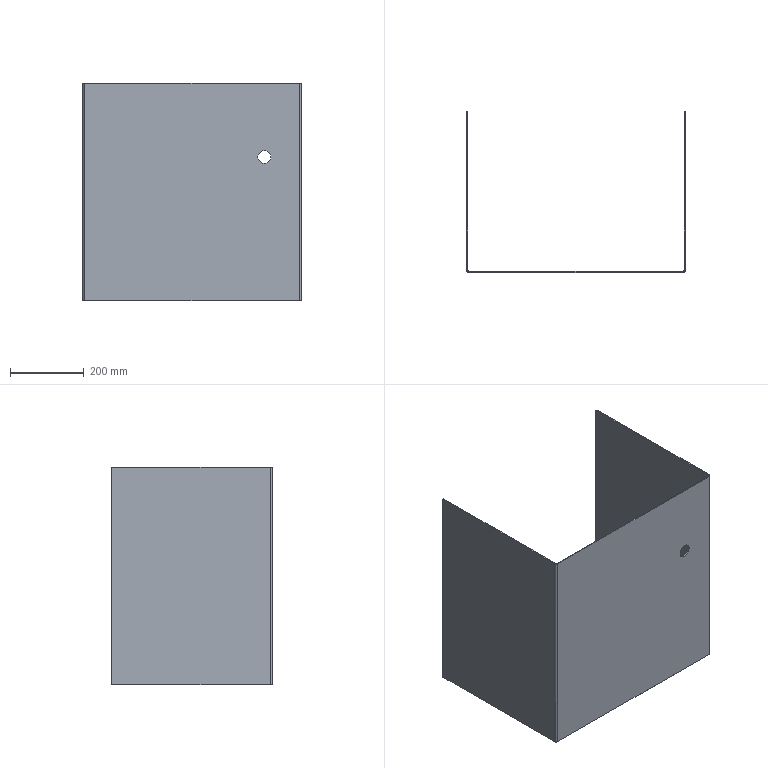Part | SolidWorks | features ICE 2, FlatPattern 1, SMBaseFlange 1, SheetMetal 1 | 1 solid | 28 faces | box 592 x 437 x 590 mm | volume 2574453 mm3 | plane 18 | cylinder 10 | commonest cylinder face diameters 6 x6 12 x2 35 x2
STEP:
#1=CARTESIAN_POINT('',(492.,0.,372.5));
#2=VERTEX_POINT('',#1);
#3=CARTESIAN_POINT('',(492.,0.,407.5));
#4=VERTEX_POINT('',#3);
#5=CARTESIAN_POINT('',(492.,0.,390.));
#6=DIRECTION('',(0.,1.,0.));
#7=DIRECTION('',(0.,0.,1.));
#8=AXIS2_PLACEMENT_3D('',#5,#6,#7);
#9=CIRCLE('',#8,17.5);
#10=EDGE_CURVE('',#2,#4,#9,.T.);
#11=ORIENTED_EDGE('',*,*,#10,.F.);
#12=CARTESIAN_POINT('',(492.,3.,372.5));
#13=VERTEX_POINT('',#12);
#14=CARTESIAN_POINT('',(492.,-7.,372.5));
#15=DIRECTION('',(0.,1.,0.));
#16=VECTOR('',#15,1000.);
#17=LINE('',#14,#16);
#18=EDGE_CURVE('',#2,#13,#17,.T.);
#19=ORIENTED_EDGE('',*,*,#18,.T.);
#20=CARTESIAN_POINT('',(492.,3.,407.5));
#21=VERTEX_POINT('',#20);
#22=CARTESIAN_POINT('',(492.,3.,390.));
#23=DIRECTION('',(0.,1.,0.));
#24=DIRECTION('',(0.,0.,1.));
#25=AXIS2_PLACEMENT_3D('',#22,#23,#24);
#26=CIRCLE('',#25,17.5);
#27=EDGE_CURVE('',#13,#21,#26,.T.);
#28=ORIENTED_EDGE('',*,*,#27,.T.);
#29=CARTESIAN_POINT('',(492.,-7.,407.5));
#30=DIRECTION('',(0.,1.,0.));
#31=VECTOR('',#30,1000.);
#32=LINE('',#29,#31);
#33=EDGE_CURVE('',#4,#21,#32,.T.);
#34=ORIENTED_EDGE('',*,*,#33,.F.);
#35=EDGE_LOOP('',(#11,#19,#28,#34));
#36=FACE_OUTER_BOUND('',#35,.T.);
#37=CARTESIAN_POINT('',(492.,-7.,390.));
#38=DIRECTION('',(0.,1.,0.));
#39=DIRECTION('',(0.,0.,1.));
#40=AXIS2_PLACEMENT_3D('',#37,#38,#39);
#41=CYLINDRICAL_SURFACE('',#40,17.5);
#42=ADVANCED_FACE('',(#36),#41,.F.);
#43=CARTESIAN_POINT('',(592.,434.,0.));
#44=VERTEX_POINT('',#43);
#45=CARTESIAN_POINT('',(592.,437.,3.));
#46=VERTEX_POINT('',#45);
#47=CARTESIAN_POINT('',(592.,434.,3.));
#48=DIRECTION('',(1.,0.,0.));
#49=DIRECTION('',(0.,0.,1.));
#50=AXIS2_PLACEMENT_3D('',#47,#48,#49);
#51=CIRCLE('',#50,3.);
#52=EDGE_CURVE('',#44,#46,#51,.T.);
#53=ORIENTED_EDGE('',*,*,#52,.T.);
#54=CARTESIAN_POINT('',(592.,437.,587.));
#55=VERTEX_POINT('',#54);
#56=CARTESIAN_POINT('',(592.,437.,590.));
#57=DIRECTION('',(0.,0.,-1.));
#58=VECTOR('',#57,1000.);
#59=LINE('',#56,#58);
#60=EDGE_CURVE('',#55,#46,#59,.T.);
#61=ORIENTED_EDGE('',*,*,#60,.F.);
#62=CARTESIAN_POINT('',(592.,434.,590.));
#63=VERTEX_POINT('',#62);
#64=CARTESIAN_POINT('',(592.,434.,587.));
#65=DIRECTION('',(1.,0.,0.));
#66=DIRECTION('',(0.,0.,1.));
#67=AXIS2_PLACEMENT_3D('',#64,#65,#66);
#68=CIRCLE('',#67,3.);
#69=EDGE_CURVE('',#55,#63,#68,.T.);
#70=ORIENTED_EDGE('',*,*,#69,.T.);
#71=CARTESIAN_POINT('',(592.,6.,590.));
#72=VERTEX_POINT('',#71);
#73=CARTESIAN_POINT('',(592.,0.,590.));
#74=DIRECTION('',(0.,1.,0.));
#75=VECTOR('',#74,1000.);
#76=LINE('',#73,#75);
#77=EDGE_CURVE('',#72,#63,#76,.T.);
#78=ORIENTED_EDGE('',*,*,#77,.F.);
#79=CARTESIAN_POINT('',(592.,6.,0.));
#80=VERTEX_POINT('',#79);
#81=CARTESIAN_POINT('',(592.,6.,590.));
#82=DIRECTION('',(0.,0.,-1.));
#83=VECTOR('',#82,1000.);
#84=LINE('',#81,#83);
#85=EDGE_CURVE('',#72,#80,#84,.T.);
#86=ORIENTED_EDGE('',*,*,#85,.T.);
#87=CARTESIAN_POINT('',(592.,0.,0.));
#88=DIRECTION('',(0.,1.,0.));
#89=VECTOR('',#88,1000.);
#90=LINE('',#87,#89);
#91=EDGE_CURVE('',#80,#44,#90,.T.);
#92=ORIENTED_EDGE('',*,*,#91,.T.);
#93=EDGE_LOOP('',(#53,#61,#70,#78,#86,#92));
#94=FACE_OUTER_BOUND('',#93,.T.);
#95=CARTESIAN_POINT('',(592.,0.,590.));
#96=DIRECTION('',(-1.,0.,0.));
#97=DIRECTION('',(0.,0.,1.));
#98=AXIS2_PLACEMENT_3D('',#95,#96,#97);
#99=PLANE('',#98);
#100=ADVANCED_FACE('',(#94),#99,.F.);
#101=CARTESIAN_POINT('',(589.,437.,587.));
#102=VERTEX_POINT('',#101);
#103=CARTESIAN_POINT('',(589.,437.,3.));
#104=VERTEX_POINT('',#103);
#105=CARTESIAN_POINT('',(589.,437.,590.));
#106=DIRECTION('',(0.,0.,-1.));
#107=VECTOR('',#106,1000.);
#108=LINE('',#105,#107);
#109=EDGE_CURVE('',#102,#104,#108,.T.);
#110=ORIENTED_EDGE('',*,*,#109,.T.);
#111=CARTESIAN_POINT('',(589.,434.,0.));
#112=VERTEX_POINT('',#111);
#113=CARTESIAN_POINT('',(589.,434.,3.));
#114=DIRECTION('',(1.,0.,0.));
#115=DIRECTION('',(0.,0.,1.));
#116=AXIS2_PLACEMENT_3D('',#113,#114,#115);
#117=CIRCLE('',#116,3.);
#118=EDGE_CURVE('',#112,#104,#117,.T.);
#119=ORIENTED_EDGE('',*,*,#118,.F.);
#120=CARTESIAN_POINT('',(589.,6.,0.));
#121=VERTEX_POINT('',#120);
#122=CARTESIAN_POINT('',(589.,0.,0.));
#123=DIRECTION('',(0.,1.,0.));
#124=VECTOR('',#123,1000.);
#125=LINE('',#122,#124);
#126=EDGE_CURVE('',#121,#112,#125,.T.);
#127=ORIENTED_EDGE('',*,*,#126,.F.);
#128=CARTESIAN_POINT('',(589.,6.,590.));
#129=VERTEX_POINT('',#128);
#130=CARTESIAN_POINT('',(589.,6.,590.));
#131=DIRECTION('',(0.,0.,-1.));
#132=VECTOR('',#131,1000.);
#133=LINE('',#130,#132);
#134=EDGE_CURVE('',#129,#121,#133,.T.);
#135=ORIENTED_EDGE('',*,*,#134,.F.);
#136=CARTESIAN_POINT('',(589.,434.,590.));
#137=VERTEX_POINT('',#136);
#138=CARTESIAN_POINT('',(589.,0.,590.));
#139=DIRECTION('',(0.,1.,0.));
#140=VECTOR('',#139,1000.);
#141=LINE('',#138,#140);
#142=EDGE_CURVE('',#129,#137,#141,.T.);
#143=ORIENTED_EDGE('',*,*,#142,.T.);
#144=CARTESIAN_POINT('',(589.,434.,587.));
#145=DIRECTION('',(1.,0.,0.));
#146=DIRECTION('',(0.,0.,1.));
#147=AXIS2_PLACEMENT_3D('',#144,#145,#146);
#148=CIRCLE('',#147,3.);
#149=EDGE_CURVE('',#102,#137,#148,.T.);
#150=ORIENTED_EDGE('',*,*,#149,.F.);
#151=EDGE_LOOP('',(#110,#119,#127,#135,#143,#150));
#152=FACE_OUTER_BOUND('',#151,.T.);
#153=CARTESIAN_POINT('',(589.,0.,590.));
#154=DIRECTION('',(-1.,0.,0.));
#155=DIRECTION('',(0.,0.,1.));
#156=AXIS2_PLACEMENT_3D('',#153,#154,#155);
#157=PLANE('',#156);
#158=ADVANCED_FACE('',(#152),#157,.T.);
#159=ORIENTED_EDGE('',*,*,#60,.T.);
#160=CARTESIAN_POINT('',(589.,437.,3.));
#161=DIRECTION('',(1.,0.,0.));
#162=VECTOR('',#161,1000.);
#163=LINE('',#160,#162);
#164=EDGE_CURVE('',#104,#46,#163,.T.);
#165=ORIENTED_EDGE('',*,*,#164,.F.);
#166=ORIENTED_EDGE('',*,*,#109,.F.);
#167=CARTESIAN_POINT('',(589.,437.,587.));
#168=DIRECTION('',(1.,0.,0.));
#169=VECTOR('',#168,1000.);
#170=LINE('',#167,#169);
#171=EDGE_CURVE('',#102,#55,#170,.T.);
#172=ORIENTED_EDGE('',*,*,#171,.T.);
#173=EDGE_LOOP('',(#159,#165,#166,#172));
#174=FACE_OUTER_BOUND('',#173,.T.);
#175=CARTESIAN_POINT('',(589.,437.,590.));
#176=DIRECTION('',(0.,1.,0.));
#177=DIRECTION('',(0.,0.,1.));
#178=AXIS2_PLACEMENT_3D('',#175,#176,#177);
#179=PLANE('',#178);
#180=ADVANCED_FACE('',(#174),#179,.T.);
#181=CARTESIAN_POINT('',(3.,434.,0.));
#182=VERTEX_POINT('',#181);
#183=CARTESIAN_POINT('',(3.,6.,0.));
#184=VERTEX_POINT('',#183);
#185=CARTESIAN_POINT('',(3.,0.,0.));
#186=DIRECTION('',(0.,-1.,0.));
#187=VECTOR('',#186,1000.);
#188=LINE('',#185,#187);
#189=EDGE_CURVE('',#182,#184,#188,.T.);
#190=ORIENTED_EDGE('',*,*,#189,.F.);
#191=CARTESIAN_POINT('',(3.,437.,3.));
#192=VERTEX_POINT('',#191);
#193=CARTESIAN_POINT('',(3.,434.,3.));
#194=DIRECTION('',(-1.,0.,0.));
#195=DIRECTION('',(0.,0.,-1.));
#196=AXIS2_PLACEMENT_3D('',#193,#194,#195);
#197=CIRCLE('',#196,3.);
#198=EDGE_CURVE('',#192,#182,#197,.T.);
#199=ORIENTED_EDGE('',*,*,#198,.F.);
#200=CARTESIAN_POINT('',(3.,437.,587.));
#201=VERTEX_POINT('',#200);
#202=CARTESIAN_POINT('',(3.,437.,590.));
#203=DIRECTION('',(0.,0.,-1.));
#204=VECTOR('',#203,1000.);
#205=LINE('',#202,#204);
#206=EDGE_CURVE('',#201,#192,#205,.T.);
#207=ORIENTED_EDGE('',*,*,#206,.F.);
#208=CARTESIAN_POINT('',(3.,434.,590.));
#209=VERTEX_POINT('',#208);
#210=CARTESIAN_POINT('',(3.,434.,587.));
#211=DIRECTION('',(-1.,0.,0.));
#212=DIRECTION('',(0.,0.,-1.));
#213=AXIS2_PLACEMENT_3D('',#210,#211,#212);
#214=CIRCLE('',#213,3.);
#215=EDGE_CURVE('',#209,#201,#214,.T.);
#216=ORIENTED_EDGE('',*,*,#215,.F.);
#217=CARTESIAN_POINT('',(3.,6.,590.));
#218=VERTEX_POINT('',#217);
#219=CARTESIAN_POINT('',(3.,0.,590.));
#220=DIRECTION('',(0.,-1.,0.));
#221=VECTOR('',#220,1000.);
#222=LINE('',#219,#221);
#223=EDGE_CURVE('',#209,#218,#222,.T.);
#224=ORIENTED_EDGE('',*,*,#223,.T.);
#225=CARTESIAN_POINT('',(3.,6.,590.));
#226=DIRECTION('',(0.,0.,-1.));
#227=VECTOR('',#226,1000.);
#228=LINE('',#225,#227);
#229=EDGE_CURVE('',#218,#184,#228,.T.);
#230=ORIENTED_EDGE('',*,*,#229,.T.);
#231=EDGE_LOOP('',(#190,#199,#207,#216,#224,#230));
#232=FACE_OUTER_BOUND('',#231,.T.);
#233=CARTESIAN_POINT('',(3.,0.,590.));
#234=DIRECTION('',(1.,0.,0.));
#235=DIRECTION('',(0.,0.,-1.));
#236=AXIS2_PLACEMENT_3D('',#233,#234,#235);
#237=PLANE('',#236);
#238=ADVANCED_FACE('',(#232),#237,.T.);
#239=CARTESIAN_POINT('',(0.,437.,3.));
#240=VERTEX_POINT('',#239);
#241=CARTESIAN_POINT('',(0.,434.,0.));
#242=VERTEX_POINT('',#241);
#243=CARTESIAN_POINT('',(0.,434.,3.));
#244=DIRECTION('',(-1.,0.,0.));
#245=DIRECTION('',(0.,0.,-1.));
#246=AXIS2_PLACEMENT_3D('',#243,#244,#245);
#247=CIRCLE('',#246,3.);
#248=EDGE_CURVE('',#240,#242,#247,.T.);
#249=ORIENTED_EDGE('',*,*,#248,.T.);
#250=CARTESIAN_POINT('',(0.,6.,0.));
#251=VERTEX_POINT('',#250);
#252=CARTESIAN_POINT('',(0.,0.,0.));
#253=DIRECTION('',(0.,-1.,0.));
#254=VECTOR('',#253,1000.);
#255=LINE('',#252,#254);
#256=EDGE_CURVE('',#242,#251,#255,.T.);
#257=ORIENTED_EDGE('',*,*,#256,.T.);
#258=CARTESIAN_POINT('',(0.,6.,590.));
#259=VERTEX_POINT('',#258);
#260=CARTESIAN_POINT('',(0.,6.,590.));
#261=DIRECTION('',(0.,0.,-1.));
#262=VECTOR('',#261,1000.);
#263=LINE('',#260,#262);
#264=EDGE_CURVE('',#259,#251,#263,.T.);
#265=ORIENTED_EDGE('',*,*,#264,.F.);
#266=CARTESIAN_POINT('',(0.,434.,590.));
#267=VERTEX_POINT('',#266);
#268=CARTESIAN_POINT('',(0.,0.,590.));
#269=DIRECTION('',(0.,-1.,0.));
#270=VECTOR('',#269,1000.);
#271=LINE('',#268,#270);
#272=EDGE_CURVE('',#267,#259,#271,.T.);
#273=ORIENTED_EDGE('',*,*,#272,.F.);
#274=CARTESIAN_POINT('',(0.,437.,587.));
#275=VERTEX_POINT('',#274);
#276=CARTESIAN_POINT('',(0.,434.,587.));
#277=DIRECTION('',(-1.,0.,0.));
#278=DIRECTION('',(0.,0.,-1.));
#279=AXIS2_PLACEMENT_3D('',#276,#277,#278);
#280=CIRCLE('',#279,3.);
#281=EDGE_CURVE('',#267,#275,#280,.T.);
#282=ORIENTED_EDGE('',*,*,#281,.T.);
#283=CARTESIAN_POINT('',(0.,437.,590.));
#284=DIRECTION('',(0.,0.,-1.));
#285=VECTOR('',#284,1000.);
#286=LINE('',#283,#285);
#287=EDGE_CURVE('',#275,#240,#286,.T.);
#288=ORIENTED_EDGE('',*,*,#287,.T.);
#289=EDGE_LOOP('',(#249,#257,#265,#273,#282,#288));
#290=FACE_OUTER_BOUND('',#289,.T.);
#291=CARTESIAN_POINT('',(0.,0.,590.));
#292=DIRECTION('',(1.,0.,0.));
#293=DIRECTION('',(0.,0.,-1.));
#294=AXIS2_PLACEMENT_3D('',#291,#292,#293);
#295=PLANE('',#294);
#296=ADVANCED_FACE('',(#290),#295,.F.);
#297=ORIENTED_EDGE('',*,*,#77,.T.);
#298=CARTESIAN_POINT('',(589.,434.,590.));
#299=DIRECTION('',(1.,0.,0.));
#300=VECTOR('',#299,1000.);
#301=LINE('',#298,#300);
#302=EDGE_CURVE('',#137,#63,#301,.T.);
#303=ORIENTED_EDGE('',*,*,#302,.F.);
#304=ORIENTED_EDGE('',*,*,#142,.F.);
#305=CARTESIAN_POINT('',(589.,6.,590.));
#306=DIRECTION('',(1.,0.,0.));
#307=VECTOR('',#306,1000.);
#308=LINE('',#305,#307);
#309=EDGE_CURVE('',#129,#72,#308,.T.);
#310=ORIENTED_EDGE('',*,*,#309,.T.);
#311=EDGE_LOOP('',(#297,#303,#304,#310));
#312=FACE_OUTER_BOUND('',#311,.T.);
#313=CARTESIAN_POINT('',(586.,6.,590.));
#314=DIRECTION('',(0.,0.,1.));
#315=DIRECTION('',(1.,0.,0.));
#316=AXIS2_PLACEMENT_3D('',#313,#314,#315);
#317=PLANE('',#316);
#318=ADVANCED_FACE('',(#312),#317,.T.);
#319=CARTESIAN_POINT('',(3.,437.,3.));
#320=DIRECTION('',(-1.,0.,0.));
#321=VECTOR('',#320,1000.);
#322=LINE('',#319,#321);
#323=EDGE_CURVE('',#192,#240,#322,.T.);
#324=ORIENTED_EDGE('',*,*,#323,.T.);
#325=ORIENTED_EDGE('',*,*,#287,.F.);
#326=CARTESIAN_POINT('',(3.,437.,587.));
#327=DIRECTION('',(-1.,0.,0.));
#328=VECTOR('',#327,1000.);
#329=LINE('',#326,#328);
#330=EDGE_CURVE('',#201,#275,#329,.T.);
#331=ORIENTED_EDGE('',*,*,#330,.F.);
#332=ORIENTED_EDGE('',*,*,#206,.T.);
#333=EDGE_LOOP('',(#324,#325,#331,#332));
#334=FACE_OUTER_BOUND('',#333,.T.);
#335=CARTESIAN_POINT('',(0.,437.,590.));
#336=DIRECTION('',(0.,1.,0.));
#337=DIRECTION('',(0.,0.,1.));
#338=AXIS2_PLACEMENT_3D('',#335,#336,#337);
#339=PLANE('',#338);
#340=ADVANCED_FACE('',(#334),#339,.T.);
#341=CARTESIAN_POINT('',(0.,6.,590.));
#342=DIRECTION('',(1.,0.,0.));
#343=VECTOR('',#342,1000.);
#344=LINE('',#341,#343);
#345=EDGE_CURVE('',#259,#218,#344,.T.);
#346=ORIENTED_EDGE('',*,*,#345,.F.);
#347=CARTESIAN_POINT('',(6.,0.,590.));
#348=VERTEX_POINT('',#347);
#349=CARTESIAN_POINT('',(6.,6.,590.));
#350=DIRECTION('',(0.,0.,1.));
#351=DIRECTION('',(-1.,0.,0.));
#352=AXIS2_PLACEMENT_3D('',#349,#350,#351);
#353=CIRCLE('',#352,6.);
#354=EDGE_CURVE('',#259,#348,#353,.T.);
#355=ORIENTED_EDGE('',*,*,#354,.T.);
#356=CARTESIAN_POINT('',(6.,3.,590.));
#357=VERTEX_POINT('',#356);
#358=CARTESIAN_POINT('',(6.,3.,590.));
#359=DIRECTION('',(0.,-1.,0.));
#360=VECTOR('',#359,1000.);
#361=LINE('',#358,#360);
#362=EDGE_CURVE('',#357,#348,#361,.T.);
#363=ORIENTED_EDGE('',*,*,#362,.F.);
#364=CARTESIAN_POINT('',(6.,6.,590.));
#365=DIRECTION('',(0.,0.,1.));
#366=DIRECTION('',(1.,0.,0.));
#367=AXIS2_PLACEMENT_3D('',#364,#365,#366);
#368=CIRCLE('',#367,3.);
#369=EDGE_CURVE('',#218,#357,#368,.T.);
#370=ORIENTED_EDGE('',*,*,#369,.F.);
#371=EDGE_LOOP('',(#346,#355,#363,#370));
#372=FACE_OUTER_BOUND('',#371,.T.);
#373=CARTESIAN_POINT('',(0.,6.,590.));
#374=DIRECTION('',(0.,0.,1.));
#375=DIRECTION('',(1.,0.,0.));
#376=AXIS2_PLACEMENT_3D('',#373,#374,#375);
#377=PLANE('',#376);
#378=ADVANCED_FACE('',(#372),#377,.T.);
#379=CARTESIAN_POINT('',(3.,434.,590.));
#380=DIRECTION('',(-1.,0.,0.));
#381=VECTOR('',#380,1000.);
#382=LINE('',#379,#381);
#383=EDGE_CURVE('',#209,#267,#382,.T.);
#384=ORIENTED_EDGE('',*,*,#383,.T.);
#385=ORIENTED_EDGE('',*,*,#272,.T.);
#386=ORIENTED_EDGE('',*,*,#345,.T.);
#387=ORIENTED_EDGE('',*,*,#223,.F.);
#388=EDGE_LOOP('',(#384,#385,#386,#387));
#389=FACE_OUTER_BOUND('',#388,.T.);
#390=CARTESIAN_POINT('',(6.,3.,590.));
#391=DIRECTION('',(0.,0.,1.));
#392=DIRECTION('',(1.,0.,0.));
#393=AXIS2_PLACEMENT_3D('',#390,#391,#392);
#394=PLANE('',#393);
#395=ADVANCED_FACE('',(#389),#394,.T.);
#396=CARTESIAN_POINT('',(6.,0.,0.));
#397=VERTEX_POINT('',#396);
#398=CARTESIAN_POINT('',(6.,3.,0.));
#399=VERTEX_POINT('',#398);
#400=CARTESIAN_POINT('',(6.,0.,0.));
#401=DIRECTION('',(0.,1.,0.));
#402=VECTOR('',#401,1000.);
#403=LINE('',#400,#402);
#404=EDGE_CURVE('',#397,#399,#403,.T.);
#405=ORIENTED_EDGE('',*,*,#404,.F.);
#406=CARTESIAN_POINT('',(6.,6.,0.));
#407=DIRECTION('',(0.,0.,1.));
#408=DIRECTION('',(-1.,0.,0.));
#409=AXIS2_PLACEMENT_3D('',#406,#407,#408);
#410=CIRCLE('',#409,6.);
#411=EDGE_CURVE('',#251,#397,#410,.T.);
#412=ORIENTED_EDGE('',*,*,#411,.F.);
#413=CARTESIAN_POINT('',(3.,6.,0.));
#414=DIRECTION('',(-1.,0.,0.));
#415=VECTOR('',#414,1000.);
#416=LINE('',#413,#415);
#417=EDGE_CURVE('',#184,#251,#416,.T.);
#418=ORIENTED_EDGE('',*,*,#417,.F.);
#419=CARTESIAN_POINT('',(6.,6.,0.));
#420=DIRECTION('',(0.,0.,1.));
#421=DIRECTION('',(1.,0.,0.));
#422=AXIS2_PLACEMENT_3D('',#419,#420,#421);
#423=CIRCLE('',#422,3.);
#424=EDGE_CURVE('',#184,#399,#423,.T.);
#425=ORIENTED_EDGE('',*,*,#424,.T.);
#426=EDGE_LOOP('',(#405,#412,#418,#425));
#427=FACE_OUTER_BOUND('',#426,.T.);
#428=CARTESIAN_POINT('',(6.,0.,0.));
#429=DIRECTION('',(0.,0.,-1.));
#430=DIRECTION('',(-1.,0.,0.));
#431=AXIS2_PLACEMENT_3D('',#428,#429,#430);
#432=PLANE('',#431);
#433=ADVANCED_FACE('',(#427),#432,.T.);
#434=CARTESIAN_POINT('',(586.,0.,0.));
#435=VERTEX_POINT('',#434);
#436=CARTESIAN_POINT('',(0.,0.,0.));
#437=DIRECTION('',(1.,0.,0.));
#438=VECTOR('',#437,1000.);
#439=LINE('',#436,#438);
#440=EDGE_CURVE('',#397,#435,#439,.T.);
#441=ORIENTED_EDGE('',*,*,#440,.F.);
#442=ORIENTED_EDGE('',*,*,#404,.T.);
#443=CARTESIAN_POINT('',(586.,3.,0.));
#444=VERTEX_POINT('',#443);
#445=CARTESIAN_POINT('',(0.,3.,0.));
#446=DIRECTION('',(1.,0.,0.));
#447=VECTOR('',#446,1000.);
#448=LINE('',#445,#447);
#449=EDGE_CURVE('',#399,#444,#448,.T.);
#450=ORIENTED_EDGE('',*,*,#449,.T.);
#451=CARTESIAN_POINT('',(586.,3.,0.));
#452=DIRECTION('',(0.,-1.,0.));
#453=VECTOR('',#452,1000.);
#454=LINE('',#451,#453);
#455=EDGE_CURVE('',#444,#435,#454,.T.);
#456=ORIENTED_EDGE('',*,*,#455,.T.);
#457=EDGE_LOOP('',(#441,#442,#450,#456));
#458=FACE_OUTER_BOUND('',#457,.T.);
#459=CARTESIAN_POINT('',(3.,6.,0.));
#460=DIRECTION('',(0.,0.,-1.));
#461=DIRECTION('',(-1.,0.,0.));
#462=AXIS2_PLACEMENT_3D('',#459,#460,#461);
#463=PLANE('',#462);
#464=ADVANCED_FACE('',(#458),#463,.T.);
#465=CARTESIAN_POINT('',(586.,0.,590.));
#466=VERTEX_POINT('',#465);
#467=CARTESIAN_POINT('',(586.,3.,590.));
#468=VERTEX_POINT('',#467);
#469=CARTESIAN_POINT('',(586.,0.,590.));
#470=DIRECTION('',(0.,1.,0.));
#471=VECTOR('',#470,1000.);
#472=LINE('',#469,#471);
#473=EDGE_CURVE('',#466,#468,#472,.T.);
#474=ORIENTED_EDGE('',*,*,#473,.F.);
#475=CARTESIAN_POINT('',(586.,6.,590.));
#476=DIRECTION('',(0.,0.,1.));
#477=DIRECTION('',(-1.,0.,0.));
#478=AXIS2_PLACEMENT_3D('',#475,#476,#477);
#479=CIRCLE('',#478,6.);
#480=EDGE_CURVE('',#466,#72,#479,.T.);
#481=ORIENTED_EDGE('',*,*,#480,.T.);
#482=ORIENTED_EDGE('',*,*,#309,.F.);
#483=CARTESIAN_POINT('',(586.,6.,590.));
#484=DIRECTION('',(0.,0.,1.));
#485=DIRECTION('',(1.,0.,0.));
#486=AXIS2_PLACEMENT_3D('',#483,#484,#485);
#487=CIRCLE('',#486,3.);
#488=EDGE_CURVE('',#468,#129,#487,.T.);
#489=ORIENTED_EDGE('',*,*,#488,.F.);
#490=EDGE_LOOP('',(#474,#481,#482,#489));
#491=FACE_OUTER_BOUND('',#490,.T.);
#492=CARTESIAN_POINT('',(586.,0.,590.));
#493=DIRECTION('',(0.,0.,1.));
#494=DIRECTION('',(1.,0.,0.));
#495=AXIS2_PLACEMENT_3D('',#492,#493,#494);
#496=PLANE('',#495);
#497=ADVANCED_FACE('',(#491),#496,.T.);
#498=CARTESIAN_POINT('',(0.,0.,590.));
#499=DIRECTION('',(1.,0.,0.));
#500=VECTOR('',#499,1000.);
#501=LINE('',#498,#500);
#502=EDGE_CURVE('',#348,#466,#501,.T.);
#503=ORIENTED_EDGE('',*,*,#502,.T.);
#504=ORIENTED_EDGE('',*,*,#473,.T.);
#505=CARTESIAN_POINT('',(0.,3.,590.));
#506=DIRECTION('',(1.,0.,0.));
#507=VECTOR('',#506,1000.);
#508=LINE('',#505,#507);
#509=EDGE_CURVE('',#357,#468,#508,.T.);
#510=ORIENTED_EDGE('',*,*,#509,.F.);
#511=ORIENTED_EDGE('',*,*,#362,.T.);
#512=EDGE_LOOP('',(#503,#504,#510,#511));
#513=FACE_OUTER_BOUND('',#512,.T.);
#514=CARTESIAN_POINT('',(589.,6.,590.));
#515=DIRECTION('',(0.,0.,1.));
#516=DIRECTION('',(1.,0.,0.));
#517=AXIS2_PLACEMENT_3D('',#514,#515,#516);
#518=PLANE('',#517);
#519=ADVANCED_FACE('',(#513),#518,.T.);
#520=CARTESIAN_POINT('',(592.,6.,0.));
#521=DIRECTION('',(-1.,0.,0.));
#522=VECTOR('',#521,1000.);
#523=LINE('',#520,#522);
#524=EDGE_CURVE('',#80,#121,#523,.T.);
#525=ORIENTED_EDGE('',*,*,#524,.F.);
#526=CARTESIAN_POINT('',(586.,6.,0.));
#527=DIRECTION('',(0.,0.,1.));
#528=DIRECTION('',(-1.,0.,0.));
#529=AXIS2_PLACEMENT_3D('',#526,#527,#528);
#530=CIRCLE('',#529,6.);
#531=EDGE_CURVE('',#435,#80,#530,.T.);
#532=ORIENTED_EDGE('',*,*,#531,.F.);
#533=ORIENTED_EDGE('',*,*,#455,.F.);
#534=CARTESIAN_POINT('',(586.,6.,0.));
#535=DIRECTION('',(0.,0.,1.));
#536=DIRECTION('',(1.,0.,0.));
#537=AXIS2_PLACEMENT_3D('',#534,#535,#536);
#538=CIRCLE('',#537,3.);
#539=EDGE_CURVE('',#444,#121,#538,.T.);
#540=ORIENTED_EDGE('',*,*,#539,.T.);
#541=EDGE_LOOP('',(#525,#532,#533,#540));
#542=FACE_OUTER_BOUND('',#541,.T.);
#543=CARTESIAN_POINT('',(592.,6.,0.));
#544=DIRECTION('',(0.,0.,-1.));
#545=DIRECTION('',(-1.,0.,0.));
#546=AXIS2_PLACEMENT_3D('',#543,#544,#545);
#547=PLANE('',#546);
#548=ADVANCED_FACE('',(#542),#547,.T.);
#549=CARTESIAN_POINT('',(589.,434.,0.));
#550=DIRECTION('',(1.,0.,0.));
#551=VECTOR('',#550,1000.);
#552=LINE('',#549,#551);
#553=EDGE_CURVE('',#112,#44,#552,.T.);
#554=ORIENTED_EDGE('',*,*,#553,.T.);
#555=ORIENTED_EDGE('',*,*,#91,.F.);
#556=ORIENTED_EDGE('',*,*,#524,.T.);
#557=ORIENTED_EDGE('',*,*,#126,.T.);
#558=EDGE_LOOP('',(#554,#555,#556,#557));
#559=FACE_OUTER_BOUND('',#558,.T.);
#560=CARTESIAN_POINT('',(586.,3.,0.));
#561=DIRECTION('',(0.,0.,-1.));
#562=DIRECTION('',(-1.,0.,0.));
#563=AXIS2_PLACEMENT_3D('',#560,#561,#562);
#564=PLANE('',#563);
#565=ADVANCED_FACE('',(#559),#564,.T.);
#566=ORIENTED_EDGE('',*,*,#539,.F.);
#567=CARTESIAN_POINT('',(586.,3.,590.));
#568=DIRECTION('',(0.,0.,-1.));
#569=VECTOR('',#568,1000.);
#570=LINE('',#567,#569);
#571=EDGE_CURVE('',#468,#444,#570,.T.);
#572=ORIENTED_EDGE('',*,*,#571,.F.);
#573=ORIENTED_EDGE('',*,*,#488,.T.);
#574=ORIENTED_EDGE('',*,*,#134,.T.);
#575=EDGE_LOOP('',(#566,#572,#573,#574));
#576=FACE_OUTER_BOUND('',#575,.T.);
#577=CARTESIAN_POINT('',(586.,6.,590.));
#578=DIRECTION('',(0.,0.,-1.));
#579=DIRECTION('',(-1.,0.,0.));
#580=AXIS2_PLACEMENT_3D('',#577,#578,#579);
#581=CYLINDRICAL_SURFACE('',#580,3.);
#582=ADVANCED_FACE('',(#576),#581,.F.);
#583=CARTESIAN_POINT('',(492.,3.,390.));
#584=DIRECTION('',(0.,1.,0.));
#585=DIRECTION('',(0.,0.,1.));
#586=AXIS2_PLACEMENT_3D('',#583,#584,#585);
#587=CIRCLE('',#586,17.5);
#588=EDGE_CURVE('',#21,#13,#587,.T.);
#589=ORIENTED_EDGE('',*,*,#588,.F.);
#590=ORIENTED_EDGE('',*,*,#27,.F.);
#591=EDGE_LOOP('',(#589,#590));
#592=FACE_BOUND('',#591,.T.);
#593=ORIENTED_EDGE('',*,*,#449,.F.);
#594=CARTESIAN_POINT('',(6.,3.,590.));
#595=DIRECTION('',(0.,0.,-1.));
#596=VECTOR('',#595,1000.);
#597=LINE('',#594,#596);
#598=EDGE_CURVE('',#357,#399,#597,.T.);
#599=ORIENTED_EDGE('',*,*,#598,.F.);
#600=ORIENTED_EDGE('',*,*,#509,.T.);
#601=ORIENTED_EDGE('',*,*,#571,.T.);
#602=EDGE_LOOP('',(#593,#599,#600,#601));
#603=FACE_OUTER_BOUND('',#602,.T.);
#604=CARTESIAN_POINT('',(0.,3.,590.));
#605=DIRECTION('',(0.,1.,0.));
#606=DIRECTION('',(0.,0.,1.));
#607=AXIS2_PLACEMENT_3D('',#604,#605,#606);
#608=PLANE('',#607);
#609=ADVANCED_FACE('',(#592,#603),#608,.T.);
#610=ORIENTED_EDGE('',*,*,#424,.F.);
#611=ORIENTED_EDGE('',*,*,#229,.F.);
#612=ORIENTED_EDGE('',*,*,#369,.T.);
#613=ORIENTED_EDGE('',*,*,#598,.T.);
#614=EDGE_LOOP('',(#610,#611,#612,#613));
#615=FACE_OUTER_BOUND('',#614,.T.);
#616=CARTESIAN_POINT('',(6.,6.,590.));
#617=DIRECTION('',(0.,0.,-1.));
#618=DIRECTION('',(-1.,0.,0.));
#619=AXIS2_PLACEMENT_3D('',#616,#617,#618);
#620=CYLINDRICAL_SURFACE('',#619,3.);
#621=ADVANCED_FACE('',(#615),#620,.F.);
#622=ORIENTED_EDGE('',*,*,#411,.T.);
#623=CARTESIAN_POINT('',(6.,0.,590.));
#624=DIRECTION('',(0.,0.,-1.));
#625=VECTOR('',#624,1000.);
#626=LINE('',#623,#625);
#627=EDGE_CURVE('',#348,#397,#626,.T.);
#628=ORIENTED_EDGE('',*,*,#627,.F.);
#629=ORIENTED_EDGE('',*,*,#354,.F.);
#630=ORIENTED_EDGE('',*,*,#264,.T.);
#631=EDGE_LOOP('',(#622,#628,#629,#630));
#632=FACE_OUTER_BOUND('',#631,.T.);
#633=CARTESIAN_POINT('',(6.,6.,590.));
#634=DIRECTION('',(0.,0.,-1.));
#635=DIRECTION('',(-1.,0.,0.));
#636=AXIS2_PLACEMENT_3D('',#633,#634,#635);
#637=CYLINDRICAL_SURFACE('',#636,6.);
#638=ADVANCED_FACE('',(#632),#637,.T.);
#639=CARTESIAN_POINT('',(492.,0.,390.));
#640=DIRECTION('',(0.,1.,0.));
#641=DIRECTION('',(0.,0.,1.));
#642=AXIS2_PLACEMENT_3D('',#639,#640,#641);
#643=CIRCLE('',#642,17.5);
#644=EDGE_CURVE('',#4,#2,#643,.T.);
#645=ORIENTED_EDGE('',*,*,#644,.T.);
#646=ORIENTED_EDGE('',*,*,#10,.T.);
#647=EDGE_LOOP('',(#645,#646));
#648=FACE_BOUND('',#647,.T.);
#649=ORIENTED_EDGE('',*,*,#440,.T.);
#650=CARTESIAN_POINT('',(586.,0.,590.));
#651=DIRECTION('',(0.,0.,-1.));
#652=VECTOR('',#651,1000.);
#653=LINE('',#650,#652);
#654=EDGE_CURVE('',#466,#435,#653,.T.);
#655=ORIENTED_EDGE('',*,*,#654,.F.);
#656=ORIENTED_EDGE('',*,*,#502,.F.);
#657=ORIENTED_EDGE('',*,*,#627,.T.);
#658=EDGE_LOOP('',(#649,#655,#656,#657));
#659=FACE_OUTER_BOUND('',#658,.T.);
#660=CARTESIAN_POINT('',(0.,0.,590.));
#661=DIRECTION('',(0.,1.,0.));
#662=DIRECTION('',(0.,0.,1.));
#663=AXIS2_PLACEMENT_3D('',#660,#661,#662);
#664=PLANE('',#663);
#665=ADVANCED_FACE('',(#648,#659),#664,.F.);
#666=ORIENTED_EDGE('',*,*,#531,.T.);
#667=ORIENTED_EDGE('',*,*,#85,.F.);
#668=ORIENTED_EDGE('',*,*,#480,.F.);
#669=ORIENTED_EDGE('',*,*,#654,.T.);
#670=EDGE_LOOP('',(#666,#667,#668,#669));
#671=FACE_OUTER_BOUND('',#670,.T.);
#672=CARTESIAN_POINT('',(586.,6.,590.));
#673=DIRECTION('',(0.,0.,-1.));
#674=DIRECTION('',(-1.,0.,0.));
#675=AXIS2_PLACEMENT_3D('',#672,#673,#674);
#676=CYLINDRICAL_SURFACE('',#675,6.);
#677=ADVANCED_FACE('',(#671),#676,.T.);
#678=ORIENTED_EDGE('',*,*,#256,.F.);
#679=CARTESIAN_POINT('',(3.,434.,0.));
#680=DIRECTION('',(-1.,0.,0.));
#681=VECTOR('',#680,1000.);
#682=LINE('',#679,#681);
#683=EDGE_CURVE('',#182,#242,#682,.T.);
#684=ORIENTED_EDGE('',*,*,#683,.F.);
#685=ORIENTED_EDGE('',*,*,#189,.T.);
#686=ORIENTED_EDGE('',*,*,#417,.T.);
#687=EDGE_LOOP('',(#678,#684,#685,#686));
#688=FACE_OUTER_BOUND('',#687,.T.);
#689=CARTESIAN_POINT('',(586.,6.,0.));
#690=DIRECTION('',(0.,0.,1.));
#691=DIRECTION('',(1.,0.,0.));
#692=AXIS2_PLACEMENT_3D('',#689,#690,#691);
#693=PLANE('',#692);
#694=ADVANCED_FACE('',(#688),#693,.F.);
#695=ORIENTED_EDGE('',*,*,#18,.F.);
#696=ORIENTED_EDGE('',*,*,#644,.F.);
#697=ORIENTED_EDGE('',*,*,#33,.T.);
#698=ORIENTED_EDGE('',*,*,#588,.T.);
#699=EDGE_LOOP('',(#695,#696,#697,#698));
#700=FACE_OUTER_BOUND('',#699,.T.);
#701=CARTESIAN_POINT('',(492.,-7.,390.));
#702=DIRECTION('',(0.,1.,0.));
#703=DIRECTION('',(0.,0.,1.));
#704=AXIS2_PLACEMENT_3D('',#701,#702,#703);
#705=CYLINDRICAL_SURFACE('',#704,17.5);
#706=ADVANCED_FACE('',(#700),#705,.F.);
#707=ORIENTED_EDGE('',*,*,#215,.T.);
#708=ORIENTED_EDGE('',*,*,#330,.T.);
#709=ORIENTED_EDGE('',*,*,#281,.F.);
#710=ORIENTED_EDGE('',*,*,#383,.F.);
#711=EDGE_LOOP('',(#707,#708,#709,#710));
#712=FACE_OUTER_BOUND('',#711,.T.);
#713=CARTESIAN_POINT('',(3.,434.,587.));
#714=DIRECTION('',(1.,0.,0.));
#715=DIRECTION('',(0.,0.,-1.));
#716=AXIS2_PLACEMENT_3D('',#713,#714,#715);
#717=CYLINDRICAL_SURFACE('',#716,3.);
#718=ADVANCED_FACE('',(#712),#717,.T.);
#719=ORIENTED_EDGE('',*,*,#149,.T.);
#720=ORIENTED_EDGE('',*,*,#302,.T.);
#721=ORIENTED_EDGE('',*,*,#69,.F.);
#722=ORIENTED_EDGE('',*,*,#171,.F.);
#723=EDGE_LOOP('',(#719,#720,#721,#722));
#724=FACE_OUTER_BOUND('',#723,.T.);
#725=CARTESIAN_POINT('',(589.,434.,587.));
#726=DIRECTION('',(-1.,0.,0.));
#727=DIRECTION('',(0.,0.,1.));
#728=AXIS2_PLACEMENT_3D('',#725,#726,#727);
#729=CYLINDRICAL_SURFACE('',#728,3.);
#730=ADVANCED_FACE('',(#724),#729,.T.);
#731=ORIENTED_EDGE('',*,*,#198,.T.);
#732=ORIENTED_EDGE('',*,*,#683,.T.);
#733=ORIENTED_EDGE('',*,*,#248,.F.);
#734=ORIENTED_EDGE('',*,*,#323,.F.);
#735=EDGE_LOOP('',(#731,#732,#733,#734));
#736=FACE_OUTER_BOUND('',#735,.T.);
#737=CARTESIAN_POINT('',(3.,434.,3.));
#738=DIRECTION('',(1.,0.,0.));
#739=DIRECTION('',(0.,0.,-1.));
#740=AXIS2_PLACEMENT_3D('',#737,#738,#739);
#741=CYLINDRICAL_SURFACE('',#740,3.);
#742=ADVANCED_FACE('',(#736),#741,.T.);
#743=ORIENTED_EDGE('',*,*,#118,.T.);
#744=ORIENTED_EDGE('',*,*,#164,.T.);
#745=ORIENTED_EDGE('',*,*,#52,.F.);
#746=ORIENTED_EDGE('',*,*,#553,.F.);
#747=EDGE_LOOP('',(#743,#744,#745,#746));
#748=FACE_OUTER_BOUND('',#747,.T.);
#749=CARTESIAN_POINT('',(589.,434.,3.));
#750=DIRECTION('',(-1.,0.,0.));
#751=DIRECTION('',(0.,0.,1.));
#752=AXIS2_PLACEMENT_3D('',#749,#750,#751);
#753=CYLINDRICAL_SURFACE('',#752,3.);
#754=ADVANCED_FACE('',(#748),#753,.T.);
#755=CLOSED_SHELL('',(#42,#100,#158,#180,#238,#296,#318,#340,#378,#395,#433,#464,#497,#519,#548,#565,#582,#609,#621,#638,#665,#677,#694,#706,#718,#730,#742,#754));
#756=MANIFOLD_SOLID_BREP('',#755);
#757=CARTESIAN_POINT('',(0.,0.,0.));
#758=DIRECTION('',(0.,0.,1.));
#759=DIRECTION('',(1.,0.,0.));
#760=AXIS2_PLACEMENT_3D('',#757,#758,#759);
#761=(LENGTH_UNIT()NAMED_UNIT(*)SI_UNIT(.MILLI.,.METRE.));
#762=UNCERTAINTY_MEASURE_WITH_UNIT(LENGTH_MEASURE(0.00001),#761,'','');
#763=(NAMED_UNIT(*)PLANE_ANGLE_UNIT()SI_UNIT($,.RADIAN.));
#764=(NAMED_UNIT(*)SI_UNIT($,.STERADIAN.)SOLID_ANGLE_UNIT());
#765=(GEOMETRIC_REPRESENTATION_CONTEXT(3)GLOBAL_UNCERTAINTY_ASSIGNED_CONTEXT((#762))GLOBAL_UNIT_ASSIGNED_CONTEXT((#761,#763,#764))REPRESENTATION_CONTEXT('',''));
#766=ADVANCED_BREP_SHAPE_REPRESENTATION('',(#756,#760),#765);